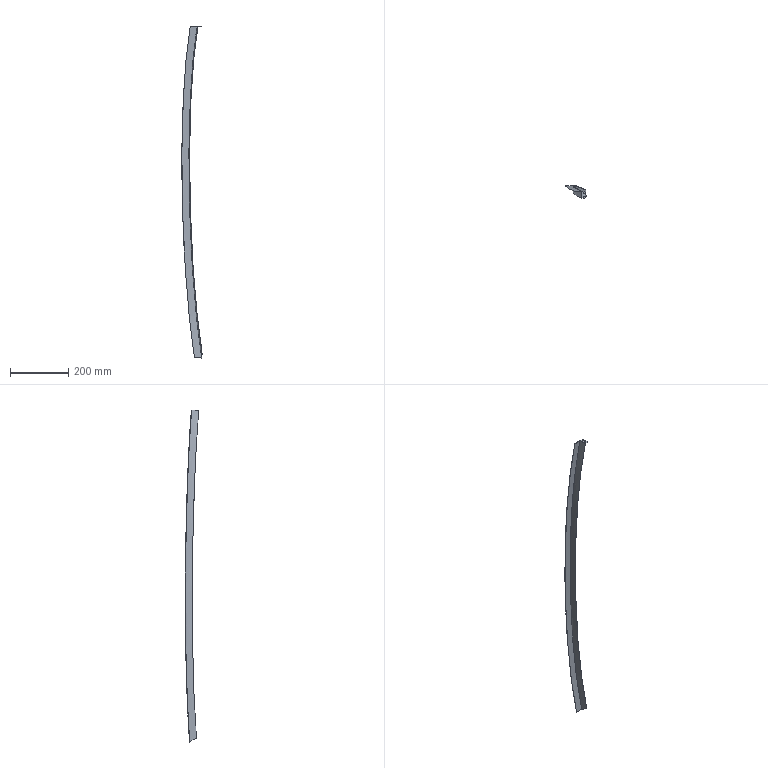Part | SolidWorks | features BaseBody 2 | 2 solids | 19 faces | box 69.762 x 45.708 x 1140 mm | volume 41473 mm3 | plane 10 | spline 5 | cylinder 4 | commonest cylinder face diameters 3.2 x4
STEP:
#1=CARTESIAN_POINT('',(-229.182,136.394,-526.751));
#2=VERTEX_POINT('',#1);
#3=CARTESIAN_POINT('',(-230.802,159.266,-540.095));
#4=VERTEX_POINT('',#3);
#5=CARTESIAN_POINT('',(-229.182,136.394,-526.751));
#6=DIRECTION('',(-0.06105,0.8621,-0.503));
#7=VECTOR('',#6,1000.);
#8=LINE('',#5,#7);
#9=EDGE_CURVE('',#2,#4,#8,.T.);
#10=ORIENTED_EDGE('',*,*,#9,.T.);
#11=CARTESIAN_POINT('',(-255.331,159.266,-540.095));
#12=VERTEX_POINT('',#11);
#13=CARTESIAN_POINT('',(-241.927,159.266,-540.095));
#14=DIRECTION('',(-1.,0.,0.));
#15=VECTOR('',#14,1000.);
#16=LINE('',#13,#15);
#17=EDGE_CURVE('',#4,#12,#16,.T.);
#18=ORIENTED_EDGE('',*,*,#17,.T.);
#19=CARTESIAN_POINT('',(-255.331,159.698,-540.347));
#20=VERTEX_POINT('',#19);
#21=CARTESIAN_POINT('',(-255.331,159.482,-540.221));
#22=DIRECTION('',(0.,-0.8638,0.5039));
#23=VECTOR('',#22,1000.);
#24=LINE('',#21,#23);
#25=EDGE_CURVE('',#20,#12,#24,.T.);
#26=ORIENTED_EDGE('',*,*,#25,.F.);
#27=CARTESIAN_POINT('',(-230.802,159.698,-540.347));
#28=VERTEX_POINT('',#27);
#29=CARTESIAN_POINT('',(-241.927,159.698,-540.347));
#30=DIRECTION('',(1.,0.,0.));
#31=VECTOR('',#30,1000.);
#32=LINE('',#29,#31);
#33=EDGE_CURVE('',#20,#28,#32,.T.);
#34=ORIENTED_EDGE('',*,*,#33,.T.);
#35=CARTESIAN_POINT('',(-230.303,159.292,-540.11));
#36=VERTEX_POINT('',#35);
#37=CARTESIAN_POINT('',(-230.802,159.698,-540.347));
#38=CARTESIAN_POINT('',(-230.739,159.698,-540.347));
#39=CARTESIAN_POINT('',(-230.614,159.677,-540.335));
#40=CARTESIAN_POINT('',(-230.454,159.59,-540.284));
#41=CARTESIAN_POINT('',(-230.34,159.458,-540.207));
#42=CARTESIAN_POINT('',(-230.307,159.349,-540.143));
#43=CARTESIAN_POINT('',(-230.303,159.292,-540.11));
#44=B_SPLINE_CURVE_WITH_KNOTS('',3,(#37,#38,#39,#40,#41,#42,#43),.UNSPECIFIED.,.F.,.F.,(4,1,1,1,4),(0.,0.0001877,0.0003754,0.0005631,0.0007508),.UNSPECIFIED.);
#45=EDGE_CURVE('',#28,#36,#44,.T.);
#46=ORIENTED_EDGE('',*,*,#45,.T.);
#47=CARTESIAN_POINT('',(-228.683,136.42,-526.767));
#48=VERTEX_POINT('',#47);
#49=CARTESIAN_POINT('',(-230.303,159.292,-540.11));
#50=DIRECTION('',(0.06105,-0.8621,0.503));
#51=VECTOR('',#50,1000.);
#52=LINE('',#49,#51);
#53=EDGE_CURVE('',#36,#48,#52,.T.);
#54=ORIENTED_EDGE('',*,*,#53,.T.);
#55=CARTESIAN_POINT('',(-228.933,136.407,-526.759));
#56=DIRECTION('',(0.9981,0.05273,-0.03076));
#57=VECTOR('',#56,1000.);
#58=LINE('',#55,#57);
#59=EDGE_CURVE('',#2,#48,#58,.T.);
#60=ORIENTED_EDGE('',*,*,#59,.F.);
#61=EDGE_LOOP('',(#10,#18,#26,#34,#46,#54,#60));
#62=FACE_OUTER_BOUND('',#61,.T.);
#63=CARTESIAN_POINT('',(-255.331,136.254,-526.67));
#64=DIRECTION('',(0.,-0.5039,-0.8638));
#65=DIRECTION('',(0.,0.8638,-0.5039));
#66=AXIS2_PLACEMENT_3D('',#63,#64,#65);
#67=PLANE('',#66);
#68=ADVANCED_FACE('',(#62),#67,.T.);
#69=ORIENTED_EDGE('',*,*,#17,.F.);
#70=CARTESIAN_POINT('',(-245.765,152.9,599.5));
#71=VERTEX_POINT('',#70);
#72=CARTESIAN_POINT('',(-230.802,159.266,-540.095));
#73=CARTESIAN_POINT('',(-278.517,182.395,-221.327));
#74=CARTESIAN_POINT('',(-291.651,175.741,308.037));
#75=CARTESIAN_POINT('',(-245.765,152.9,599.5));
#76=B_SPLINE_CURVE_WITH_KNOTS('',3,(#72,#73,#74,#75),.UNSPECIFIED.,.F.,.F.,(4,4),(0.,1.),.UNSPECIFIED.);
#77=EDGE_CURVE('',#4,#71,#76,.T.);
#78=ORIENTED_EDGE('',*,*,#77,.T.);
#79=CARTESIAN_POINT('',(-269.86,152.9,599.5));
#80=VERTEX_POINT('',#79);
#81=CARTESIAN_POINT('',(-257.812,152.9,599.5));
#82=DIRECTION('',(-1.,0.,0.));
#83=VECTOR('',#82,1000.);
#84=LINE('',#81,#83);
#85=EDGE_CURVE('',#71,#80,#84,.T.);
#86=ORIENTED_EDGE('',*,*,#85,.T.);
#87=CARTESIAN_POINT('',(-269.86,152.9,599.5));
#88=CARTESIAN_POINT('',(-315.891,175.741,308.037));
#89=CARTESIAN_POINT('',(-302.902,182.395,-221.327));
#90=CARTESIAN_POINT('',(-255.331,159.266,-540.095));
#91=B_SPLINE_CURVE_WITH_KNOTS('',3,(#87,#88,#89,#90),.UNSPECIFIED.,.F.,.F.,(4,4),(0.,1.),.UNSPECIFIED.);
#92=EDGE_CURVE('',#80,#12,#91,.T.);
#93=ORIENTED_EDGE('',*,*,#92,.T.);
#94=EDGE_LOOP('',(#69,#78,#86,#93));
#95=FACE_OUTER_BOUND('',#94,.T.);
#96=CARTESIAN_POINT('',(-245.524,152.9,599.5));
#97=CARTESIAN_POINT('',(-291.408,175.741,308.037));
#98=CARTESIAN_POINT('',(-278.273,182.395,-221.327));
#99=CARTESIAN_POINT('',(-230.556,159.266,-540.095));
#100=CARTESIAN_POINT('',(-245.604,152.9,599.5));
#101=CARTESIAN_POINT('',(-291.489,175.741,308.037));
#102=CARTESIAN_POINT('',(-278.355,182.395,-221.327));
#103=CARTESIAN_POINT('',(-230.638,159.266,-540.095));
#104=CARTESIAN_POINT('',(-245.685,152.9,599.5));
#105=CARTESIAN_POINT('',(-291.57,175.741,308.037));
#106=CARTESIAN_POINT('',(-278.436,182.395,-221.327));
#107=CARTESIAN_POINT('',(-230.72,159.266,-540.095));
#108=CARTESIAN_POINT('',(-245.765,152.9,599.5));
#109=CARTESIAN_POINT('',(-291.651,175.741,308.037));
#110=CARTESIAN_POINT('',(-278.517,182.395,-221.327));
#111=CARTESIAN_POINT('',(-230.802,159.266,-540.095));
#112=CARTESIAN_POINT('',(-247.773,152.9,599.5));
#113=CARTESIAN_POINT('',(-293.671,175.741,308.037));
#114=CARTESIAN_POINT('',(-280.549,182.395,-221.327));
#115=CARTESIAN_POINT('',(-232.846,159.266,-540.095));
#116=CARTESIAN_POINT('',(-251.789,152.9,599.5));
#117=CARTESIAN_POINT('',(-297.711,175.741,308.037));
#118=CARTESIAN_POINT('',(-284.614,182.395,-221.327));
#119=CARTESIAN_POINT('',(-236.934,159.266,-540.095));
#120=CARTESIAN_POINT('',(-257.812,152.9,599.5));
#121=CARTESIAN_POINT('',(-303.771,175.741,308.037));
#122=CARTESIAN_POINT('',(-290.71,182.395,-221.327));
#123=CARTESIAN_POINT('',(-243.067,159.266,-540.095));
#124=CARTESIAN_POINT('',(-263.836,152.9,599.5));
#125=CARTESIAN_POINT('',(-309.831,175.741,308.037));
#126=CARTESIAN_POINT('',(-296.806,182.395,-221.327));
#127=CARTESIAN_POINT('',(-249.199,159.266,-540.095));
#128=CARTESIAN_POINT('',(-267.852,152.9,599.5));
#129=CARTESIAN_POINT('',(-313.871,175.741,308.037));
#130=CARTESIAN_POINT('',(-300.87,182.395,-221.327));
#131=CARTESIAN_POINT('',(-253.287,159.266,-540.095));
#132=CARTESIAN_POINT('',(-269.86,152.9,599.5));
#133=CARTESIAN_POINT('',(-315.891,175.741,308.037));
#134=CARTESIAN_POINT('',(-302.902,182.395,-221.327));
#135=CARTESIAN_POINT('',(-255.331,159.266,-540.095));
#136=CARTESIAN_POINT('',(-269.94,152.9,599.5));
#137=CARTESIAN_POINT('',(-315.971,175.741,308.037));
#138=CARTESIAN_POINT('',(-302.983,182.395,-221.327));
#139=CARTESIAN_POINT('',(-255.413,159.266,-540.095));
#140=CARTESIAN_POINT('',(-270.021,152.9,599.5));
#141=CARTESIAN_POINT('',(-316.052,175.741,308.037));
#142=CARTESIAN_POINT('',(-303.065,182.395,-221.327));
#143=CARTESIAN_POINT('',(-255.495,159.266,-540.095));
#144=CARTESIAN_POINT('',(-270.101,152.9,599.5));
#145=CARTESIAN_POINT('',(-316.133,175.741,308.037));
#146=CARTESIAN_POINT('',(-303.146,182.395,-221.327));
#147=CARTESIAN_POINT('',(-255.577,159.266,-540.095));
#148=B_SPLINE_SURFACE_WITH_KNOTS('',3,3,((#96,#97,#98,#99),(#100,#101,#102,#103),(#104,#105,#106,#107),(#108,#109,#110,#111),(#112,#113,#114,#115),(#116,#117,#118,#119),(#120,#121,#122,#123),(#124,#125,#126,#127),(#128,#129,#130,#131),(#132,#133,#134,#135),(#136,#137,#138,#139),(#140,#141,#142,#143),(#144,#145,#146,#147)),.UNSPECIFIED.,.F.,.F.,.F.,(4,3,1,1,1,3,4),(4,4),(0.7539,0.7562,0.816,0.8757,0.9354,0.9951,0.9975),(0.,1.),.UNSPECIFIED.);
#149=ADVANCED_FACE('',(#95),#148,.T.);
#150=ORIENTED_EDGE('',*,*,#9,.F.);
#151=CARTESIAN_POINT('',(-243.797,128.416,599.5));
#152=VERTEX_POINT('',#151);
#153=CARTESIAN_POINT('',(-229.182,136.394,-526.751));
#154=CARTESIAN_POINT('',(-276.782,158.986,-212.431));
#155=CARTESIAN_POINT('',(-289.799,151.794,312.485));
#156=CARTESIAN_POINT('',(-243.797,128.416,599.5));
#157=B_SPLINE_CURVE_WITH_KNOTS('',3,(#153,#154,#155,#156),.UNSPECIFIED.,.F.,.F.,(4,4),(0.,1.),.UNSPECIFIED.);
#158=EDGE_CURVE('',#2,#152,#157,.T.);
#159=ORIENTED_EDGE('',*,*,#158,.T.);
#160=CARTESIAN_POINT('',(-245.266,152.431,599.5));
#161=VERTEX_POINT('',#160);
#162=CARTESIAN_POINT('',(-245.266,152.431,599.5));
#163=DIRECTION('',(-0.06105,0.9981,0.));
#164=VECTOR('',#163,1000.);
#165=LINE('',#162,#164);
#166=EDGE_CURVE('',#152,#161,#165,.T.);
#167=ORIENTED_EDGE('',*,*,#166,.T.);
#168=CARTESIAN_POINT('',(-245.266,152.431,599.5));
#169=CARTESIAN_POINT('',(-245.27,152.49,599.5));
#170=CARTESIAN_POINT('',(-245.299,152.612,599.5));
#171=CARTESIAN_POINT('',(-245.412,152.771,599.5));
#172=CARTESIAN_POINT('',(-245.577,152.877,599.5));
#173=CARTESIAN_POINT('',(-245.703,152.9,599.5));
#174=CARTESIAN_POINT('',(-245.765,152.9,599.5));
#175=B_SPLINE_CURVE_WITH_KNOTS('',3,(#168,#169,#170,#171,#172,#173,#174),.UNSPECIFIED.,.F.,.F.,(4,1,1,1,4),(0.,0.0001877,0.0003755,0.0005632,0.000751),.UNSPECIFIED.);
#176=EDGE_CURVE('',#161,#71,#175,.T.);
#177=ORIENTED_EDGE('',*,*,#176,.T.);
#178=ORIENTED_EDGE('',*,*,#77,.F.);
#179=EDGE_LOOP('',(#150,#159,#167,#177,#178));
#180=FACE_OUTER_BOUND('',#179,.T.);
#181=CARTESIAN_POINT('',(-243.782,128.169,599.5));
#182=CARTESIAN_POINT('',(-289.783,151.553,312.529));
#183=CARTESIAN_POINT('',(-276.766,158.751,-212.342));
#184=CARTESIAN_POINT('',(-229.166,136.165,-526.618));
#185=CARTESIAN_POINT('',(-243.787,128.251,599.5));
#186=CARTESIAN_POINT('',(-289.789,151.633,312.514));
#187=CARTESIAN_POINT('',(-276.771,158.829,-212.372));
#188=CARTESIAN_POINT('',(-229.171,136.241,-526.662));
#189=CARTESIAN_POINT('',(-243.792,128.334,599.5));
#190=CARTESIAN_POINT('',(-289.794,151.714,312.499));
#191=CARTESIAN_POINT('',(-276.776,158.907,-212.402));
#192=CARTESIAN_POINT('',(-229.177,136.317,-526.707));
#193=CARTESIAN_POINT('',(-243.797,128.416,599.5));
#194=CARTESIAN_POINT('',(-289.799,151.794,312.485));
#195=CARTESIAN_POINT('',(-276.782,158.986,-212.431));
#196=CARTESIAN_POINT('',(-229.182,136.394,-526.751));
#197=CARTESIAN_POINT('',(-243.92,130.419,599.5));
#198=CARTESIAN_POINT('',(-289.924,153.747,312.125));
#199=CARTESIAN_POINT('',(-276.91,160.888,-213.152));
#200=CARTESIAN_POINT('',(-229.313,138.246,-527.832));
#201=CARTESIAN_POINT('',(-244.164,134.421,599.5));
#202=CARTESIAN_POINT('',(-290.175,157.65,311.404));
#203=CARTESIAN_POINT('',(-277.166,164.693,-214.593));
#204=CARTESIAN_POINT('',(-229.576,141.952,-529.994));
#205=CARTESIAN_POINT('',(-244.531,140.421,599.5));
#206=CARTESIAN_POINT('',(-290.551,163.505,310.322));
#207=CARTESIAN_POINT('',(-277.551,170.402,-216.757));
#208=CARTESIAN_POINT('',(-229.97,147.515,-533.24));
#209=CARTESIAN_POINT('',(-244.898,146.422,599.5));
#210=CARTESIAN_POINT('',(-290.927,169.359,309.24));
#211=CARTESIAN_POINT('',(-277.936,176.11,-218.92));
#212=CARTESIAN_POINT('',(-230.364,153.077,-536.485));
#213=CARTESIAN_POINT('',(-245.143,150.426,599.5));
#214=CARTESIAN_POINT('',(-291.178,173.264,308.52));
#215=CARTESIAN_POINT('',(-278.193,179.915,-220.361));
#216=CARTESIAN_POINT('',(-230.626,156.782,-538.646));
#217=CARTESIAN_POINT('',(-245.27,152.49,599.5));
#218=CARTESIAN_POINT('',(-291.307,175.275,308.149));
#219=CARTESIAN_POINT('',(-278.325,181.873,-221.103));
#220=CARTESIAN_POINT('',(-230.761,158.688,-539.758));
#221=CARTESIAN_POINT('',(-245.299,152.612,599.5));
#222=CARTESIAN_POINT('',(-291.329,175.392,308.128));
#223=CARTESIAN_POINT('',(-278.34,181.986,-221.144));
#224=CARTESIAN_POINT('',(-230.768,158.795,-539.82));
#225=CARTESIAN_POINT('',(-245.412,152.771,599.5));
#226=CARTESIAN_POINT('',(-291.408,175.55,308.098));
#227=CARTESIAN_POINT('',(-278.385,182.143,-221.205));
#228=CARTESIAN_POINT('',(-230.779,158.951,-539.911));
#229=CARTESIAN_POINT('',(-245.577,152.877,599.5));
#230=CARTESIAN_POINT('',(-291.522,175.672,308.068));
#231=CARTESIAN_POINT('',(-278.447,182.281,-221.265));
#232=CARTESIAN_POINT('',(-230.79,159.106,-540.002));
#233=CARTESIAN_POINT('',(-245.703,152.9,599.5));
#234=CARTESIAN_POINT('',(-291.608,175.723,308.047));
#235=CARTESIAN_POINT('',(-278.494,182.359,-221.306));
#236=CARTESIAN_POINT('',(-230.798,159.212,-540.063));
#237=CARTESIAN_POINT('',(-245.765,152.9,599.5));
#238=CARTESIAN_POINT('',(-291.651,175.741,308.037));
#239=CARTESIAN_POINT('',(-278.517,182.395,-221.327));
#240=CARTESIAN_POINT('',(-230.802,159.266,-540.095));
#241=B_SPLINE_SURFACE_WITH_KNOTS('',3,3,((#181,#182,#183,#184),(#185,#186,#187,#188),(#189,#190,#191,#192),(#193,#194,#195,#196),(#197,#198,#199,#200),(#201,#202,#203,#204),(#205,#206,#207,#208),(#209,#210,#211,#212),(#213,#214,#215,#216),(#217,#218,#219,#220),(#221,#222,#223,#224),(#225,#226,#227,#228),(#229,#230,#231,#232),(#233,#234,#235,#236),(#237,#238,#239,#240)),.UNSPECIFIED.,.F.,.F.,.F.,(4,3,1,1,1,2,1,1,1,4),(4,4),(0.5017,0.5042,0.5654,0.6266,0.6877,0.7489,0.7508,0.7526,0.7544,0.7562),(0.,1.),.UNSPECIFIED.);
#242=ADVANCED_FACE('',(#180),#241,.T.);
#243=ORIENTED_EDGE('',*,*,#33,.F.);
#244=CARTESIAN_POINT('',(-269.86,153.4,599.5));
#245=VERTEX_POINT('',#244);
#246=CARTESIAN_POINT('',(-255.331,159.698,-540.347));
#247=CARTESIAN_POINT('',(-302.902,182.85,-221.495));
#248=CARTESIAN_POINT('',(-315.891,176.218,307.953));
#249=CARTESIAN_POINT('',(-269.86,153.4,599.5));
#250=B_SPLINE_CURVE_WITH_KNOTS('',3,(#246,#247,#248,#249),.UNSPECIFIED.,.F.,.F.,(4,4),(0.,1.),.UNSPECIFIED.);
#251=EDGE_CURVE('',#20,#245,#250,.T.);
#252=ORIENTED_EDGE('',*,*,#251,.T.);
#253=CARTESIAN_POINT('',(-245.295,153.4,599.5));
#254=VERTEX_POINT('',#253);
#255=CARTESIAN_POINT('',(-243.139,153.4,599.5));
#256=DIRECTION('',(1.,0.,0.));
#257=VECTOR('',#256,1000.);
#258=LINE('',#255,#257);
#259=EDGE_CURVE('',#245,#254,#258,.T.);
#260=ORIENTED_EDGE('',*,*,#259,.T.);
#261=CARTESIAN_POINT('',(-244.796,152.931,599.5));
#262=VERTEX_POINT('',#261);
#263=CARTESIAN_POINT('',(-245.295,153.4,599.5));
#264=CARTESIAN_POINT('',(-245.232,153.4,599.5));
#265=CARTESIAN_POINT('',(-245.105,153.376,599.5));
#266=CARTESIAN_POINT('',(-244.941,153.27,599.5));
#267=CARTESIAN_POINT('',(-244.829,153.113,599.5));
#268=CARTESIAN_POINT('',(-244.799,152.991,599.5));
#269=CARTESIAN_POINT('',(-244.796,152.931,599.5));
#270=B_SPLINE_CURVE_WITH_KNOTS('',3,(#263,#264,#265,#266,#267,#268,#269),.UNSPECIFIED.,.F.,.F.,(4,1,1,1,4),(0.,0.0001877,0.0003755,0.0005632,0.000751),.UNSPECIFIED.);
#271=EDGE_CURVE('',#254,#262,#270,.T.);
#272=ORIENTED_EDGE('',*,*,#271,.T.);
#273=CARTESIAN_POINT('',(-243.298,128.447,599.5));
#274=VERTEX_POINT('',#273);
#275=CARTESIAN_POINT('',(-243.298,128.447,599.5));
#276=DIRECTION('',(0.06105,-0.9981,0.));
#277=VECTOR('',#276,1000.);
#278=LINE('',#275,#277);
#279=EDGE_CURVE('',#262,#274,#278,.T.);
#280=ORIENTED_EDGE('',*,*,#279,.T.);
#281=CARTESIAN_POINT('',(-243.298,128.447,599.5));
#282=CARTESIAN_POINT('',(-289.3,151.823,312.48));
#283=CARTESIAN_POINT('',(-276.283,159.013,-212.442));
#284=CARTESIAN_POINT('',(-228.683,136.42,-526.767));
#285=B_SPLINE_CURVE_WITH_KNOTS('',3,(#281,#282,#283,#284),.UNSPECIFIED.,.F.,.F.,(4,4),(0.,1.),.UNSPECIFIED.);
#286=EDGE_CURVE('',#274,#48,#285,.T.);
#287=ORIENTED_EDGE('',*,*,#286,.T.);
#288=ORIENTED_EDGE('',*,*,#53,.F.);
#289=ORIENTED_EDGE('',*,*,#45,.F.);
#290=EDGE_LOOP('',(#243,#252,#260,#272,#280,#287,#288,#289));
#291=FACE_OUTER_BOUND('',#290,.T.);
#292=CARTESIAN_POINT('',(-269.86,153.4,599.5));
#293=CARTESIAN_POINT('',(-315.891,176.218,307.953));
#294=CARTESIAN_POINT('',(-302.902,182.85,-221.495));
#295=CARTESIAN_POINT('',(-255.331,159.698,-540.347));
#296=CARTESIAN_POINT('',(-267.813,153.4,599.5));
#297=CARTESIAN_POINT('',(-313.844,176.218,307.953));
#298=CARTESIAN_POINT('',(-300.857,182.85,-221.495));
#299=CARTESIAN_POINT('',(-253.287,159.698,-540.347));
#300=CARTESIAN_POINT('',(-263.719,153.4,599.5));
#301=CARTESIAN_POINT('',(-309.752,176.218,307.953));
#302=CARTESIAN_POINT('',(-296.767,182.85,-221.495));
#303=CARTESIAN_POINT('',(-249.199,159.698,-540.347));
#304=CARTESIAN_POINT('',(-257.577,153.4,599.5));
#305=CARTESIAN_POINT('',(-303.614,176.218,307.953));
#306=CARTESIAN_POINT('',(-290.631,182.85,-221.495));
#307=CARTESIAN_POINT('',(-243.067,159.698,-540.347));
#308=CARTESIAN_POINT('',(-251.436,153.4,599.5));
#309=CARTESIAN_POINT('',(-297.475,176.218,307.953));
#310=CARTESIAN_POINT('',(-284.496,182.85,-221.495));
#311=CARTESIAN_POINT('',(-236.934,159.698,-540.347));
#312=CARTESIAN_POINT('',(-247.342,153.4,599.5));
#313=CARTESIAN_POINT('',(-293.383,176.218,307.953));
#314=CARTESIAN_POINT('',(-280.406,182.85,-221.495));
#315=CARTESIAN_POINT('',(-232.846,159.698,-540.347));
#316=CARTESIAN_POINT('',(-245.232,153.4,599.5));
#317=CARTESIAN_POINT('',(-291.274,176.218,307.953));
#318=CARTESIAN_POINT('',(-278.298,182.85,-221.495));
#319=CARTESIAN_POINT('',(-230.739,159.698,-540.347));
#320=CARTESIAN_POINT('',(-245.105,153.376,599.5));
#321=CARTESIAN_POINT('',(-291.148,176.195,307.957));
#322=CARTESIAN_POINT('',(-278.172,182.828,-221.487));
#323=CARTESIAN_POINT('',(-230.614,159.677,-540.335));
#324=CARTESIAN_POINT('',(-244.941,153.27,599.5));
#325=CARTESIAN_POINT('',(-290.985,176.096,307.974));
#326=CARTESIAN_POINT('',(-278.011,182.735,-221.453));
#327=CARTESIAN_POINT('',(-230.454,159.59,-540.284));
#328=CARTESIAN_POINT('',(-244.829,153.113,599.5));
#329=CARTESIAN_POINT('',(-290.873,175.947,307.999));
#330=CARTESIAN_POINT('',(-277.898,182.594,-221.402));
#331=CARTESIAN_POINT('',(-230.34,159.458,-540.207));
#332=CARTESIAN_POINT('',(-244.799,152.991,599.5));
#333=CARTESIAN_POINT('',(-290.842,175.829,308.021));
#334=CARTESIAN_POINT('',(-277.865,182.481,-221.359));
#335=CARTESIAN_POINT('',(-230.307,159.349,-540.143));
#336=CARTESIAN_POINT('',(-244.671,150.888,599.5));
#337=CARTESIAN_POINT('',(-290.71,173.774,308.402));
#338=CARTESIAN_POINT('',(-277.73,180.473,-220.597));
#339=CARTESIAN_POINT('',(-230.168,157.388,-539.));
#340=CARTESIAN_POINT('',(-244.421,146.806,599.5));
#341=CARTESIAN_POINT('',(-290.453,169.782,309.143));
#342=CARTESIAN_POINT('',(-277.467,176.572,-219.115));
#343=CARTESIAN_POINT('',(-229.898,153.578,-536.776));
#344=CARTESIAN_POINT('',(-244.047,140.687,599.5));
#345=CARTESIAN_POINT('',(-290.069,163.796,310.255));
#346=CARTESIAN_POINT('',(-277.072,170.719,-216.89));
#347=CARTESIAN_POINT('',(-229.493,147.857,-533.439));
#348=CARTESIAN_POINT('',(-243.673,134.57,599.5));
#349=CARTESIAN_POINT('',(-289.684,157.811,311.368));
#350=CARTESIAN_POINT('',(-276.677,164.865,-214.665));
#351=CARTESIAN_POINT('',(-229.088,142.136,-530.101));
#352=CARTESIAN_POINT('',(-243.423,130.489,599.5));
#353=CARTESIAN_POINT('',(-289.428,153.82,312.109));
#354=CARTESIAN_POINT('',(-276.414,160.964,-213.183));
#355=CARTESIAN_POINT('',(-228.818,138.325,-527.878));
#356=CARTESIAN_POINT('',(-243.298,128.447,599.5));
#357=CARTESIAN_POINT('',(-289.3,151.823,312.48));
#358=CARTESIAN_POINT('',(-276.283,159.013,-212.442));
#359=CARTESIAN_POINT('',(-228.683,136.42,-526.767));
#360=B_SPLINE_SURFACE_WITH_KNOTS('',3,3,((#292,#293,#294,#295),(#296,#297,#298,#299),(#300,#301,#302,#303),(#304,#305,#306,#307),(#308,#309,#310,#311),(#312,#313,#314,#315),(#316,#317,#318,#319),(#320,#321,#322,#323),(#324,#325,#326,#327),(#328,#329,#330,#331),(#332,#333,#334,#335),(#336,#337,#338,#339),(#340,#341,#342,#343),(#344,#345,#346,#347),(#348,#349,#350,#351),(#352,#353,#354,#355),(#356,#357,#358,#359)),.UNSPECIFIED.,.F.,.F.,.F.,(4,1,1,1,2,1,1,1,2,1,1,1,4),(4,4),(0.,0.0603,0.1206,0.1809,0.2412,0.2431,0.2449,0.2468,0.2486,0.3113,0.3739,0.4366,0.4993),(0.,1.),.UNSPECIFIED.);
#361=ADVANCED_FACE('',(#291),#360,.T.);
#362=ORIENTED_EDGE('',*,*,#25,.T.);
#363=ORIENTED_EDGE('',*,*,#92,.F.);
#364=CARTESIAN_POINT('',(-269.86,153.15,599.5));
#365=DIRECTION('',(0.,1.,0.));
#366=VECTOR('',#365,1000.);
#367=LINE('',#364,#366);
#368=EDGE_CURVE('',#80,#245,#367,.T.);
#369=ORIENTED_EDGE('',*,*,#368,.T.);
#370=ORIENTED_EDGE('',*,*,#251,.F.);
#371=EDGE_LOOP('',(#362,#363,#369,#370));
#372=FACE_OUTER_BOUND('',#371,.T.);
#373=CARTESIAN_POINT('',(-269.86,152.9,599.5));
#374=CARTESIAN_POINT('',(-315.891,175.741,308.037));
#375=CARTESIAN_POINT('',(-302.902,182.395,-221.327));
#376=CARTESIAN_POINT('',(-255.331,159.266,-540.095));
#377=CARTESIAN_POINT('',(-269.86,152.942,599.5));
#378=CARTESIAN_POINT('',(-315.891,175.781,308.03));
#379=CARTESIAN_POINT('',(-302.902,182.433,-221.341));
#380=CARTESIAN_POINT('',(-255.331,159.302,-540.116));
#381=CARTESIAN_POINT('',(-269.86,153.025,599.5));
#382=CARTESIAN_POINT('',(-315.891,175.86,308.016));
#383=CARTESIAN_POINT('',(-302.902,182.509,-221.369));
#384=CARTESIAN_POINT('',(-255.331,159.374,-540.158));
#385=CARTESIAN_POINT('',(-269.86,153.15,599.5));
#386=CARTESIAN_POINT('',(-315.891,175.98,307.995));
#387=CARTESIAN_POINT('',(-302.902,182.623,-221.411));
#388=CARTESIAN_POINT('',(-255.331,159.482,-540.221));
#389=CARTESIAN_POINT('',(-269.86,153.275,599.5));
#390=CARTESIAN_POINT('',(-315.891,176.099,307.974));
#391=CARTESIAN_POINT('',(-302.902,182.736,-221.453));
#392=CARTESIAN_POINT('',(-255.331,159.59,-540.284));
#393=CARTESIAN_POINT('',(-269.86,153.358,599.5));
#394=CARTESIAN_POINT('',(-315.891,176.179,307.96));
#395=CARTESIAN_POINT('',(-302.902,182.812,-221.481));
#396=CARTESIAN_POINT('',(-255.331,159.662,-540.326));
#397=CARTESIAN_POINT('',(-269.86,153.4,599.5));
#398=CARTESIAN_POINT('',(-315.891,176.218,307.953));
#399=CARTESIAN_POINT('',(-302.902,182.85,-221.495));
#400=CARTESIAN_POINT('',(-255.331,159.698,-540.347));
#401=B_SPLINE_SURFACE_WITH_KNOTS('',3,3,((#373,#374,#375,#376),(#377,#378,#379,#380),(#381,#382,#383,#384),(#385,#386,#387,#388),(#389,#390,#391,#392),(#393,#394,#395,#396),(#397,#398,#399,#400)),.UNSPECIFIED.,.F.,.F.,.F.,(4,1,1,1,4),(4,4),(0.9951,0.9963,0.9975,0.9988,1.),(0.,1.),.UNSPECIFIED.);
#402=ADVANCED_FACE('',(#372),#401,.T.);
#403=ORIENTED_EDGE('',*,*,#85,.F.);
#404=ORIENTED_EDGE('',*,*,#176,.F.);
#405=ORIENTED_EDGE('',*,*,#166,.F.);
#406=CARTESIAN_POINT('',(-243.797,128.416,599.5));
#407=DIRECTION('',(-0.9981,-0.06105,0.));
#408=VECTOR('',#407,1000.);
#409=LINE('',#406,#408);
#410=EDGE_CURVE('',#274,#152,#409,.T.);
#411=ORIENTED_EDGE('',*,*,#410,.F.);
#412=ORIENTED_EDGE('',*,*,#279,.F.);
#413=ORIENTED_EDGE('',*,*,#271,.F.);
#414=ORIENTED_EDGE('',*,*,#259,.F.);
#415=ORIENTED_EDGE('',*,*,#368,.F.);
#416=EDGE_LOOP('',(#403,#404,#405,#411,#412,#413,#414,#415));
#417=FACE_OUTER_BOUND('',#416,.T.);
#418=CARTESIAN_POINT('',(-243.139,128.266,599.5));
#419=DIRECTION('',(0.,0.,-1.));
#420=DIRECTION('',(-1.,0.,0.));
#421=AXIS2_PLACEMENT_3D('',#418,#419,#420);
#422=PLANE('',#421);
#423=ADVANCED_FACE('',(#417),#422,.F.);
#424=ORIENTED_EDGE('',*,*,#59,.T.);
#425=ORIENTED_EDGE('',*,*,#286,.F.);
#426=ORIENTED_EDGE('',*,*,#410,.T.);
#427=ORIENTED_EDGE('',*,*,#158,.F.);
#428=EDGE_LOOP('',(#424,#425,#426,#427));
#429=FACE_OUTER_BOUND('',#428,.T.);
#430=CARTESIAN_POINT('',(-243.298,128.447,599.5));
#431=CARTESIAN_POINT('',(-289.3,151.823,312.48));
#432=CARTESIAN_POINT('',(-276.283,159.013,-212.442));
#433=CARTESIAN_POINT('',(-228.683,136.42,-526.767));
#434=CARTESIAN_POINT('',(-243.34,128.444,599.5));
#435=CARTESIAN_POINT('',(-289.341,151.821,312.48));
#436=CARTESIAN_POINT('',(-276.324,159.011,-212.441));
#437=CARTESIAN_POINT('',(-228.725,136.418,-526.765));
#438=CARTESIAN_POINT('',(-243.423,128.439,599.5));
#439=CARTESIAN_POINT('',(-289.425,151.816,312.481));
#440=CARTESIAN_POINT('',(-276.407,159.007,-212.439));
#441=CARTESIAN_POINT('',(-228.808,136.413,-526.763));
#442=CARTESIAN_POINT('',(-243.548,128.431,599.5));
#443=CARTESIAN_POINT('',(-289.549,151.809,312.482));
#444=CARTESIAN_POINT('',(-276.532,159.,-212.437));
#445=CARTESIAN_POINT('',(-228.933,136.407,-526.759));
#446=CARTESIAN_POINT('',(-243.672,128.424,599.5));
#447=CARTESIAN_POINT('',(-289.674,151.802,312.483));
#448=CARTESIAN_POINT('',(-276.657,158.993,-212.434));
#449=CARTESIAN_POINT('',(-229.057,136.4,-526.755));
#450=CARTESIAN_POINT('',(-243.756,128.419,599.5));
#451=CARTESIAN_POINT('',(-289.757,151.797,312.484));
#452=CARTESIAN_POINT('',(-276.74,158.988,-212.432));
#453=CARTESIAN_POINT('',(-229.141,136.396,-526.752));
#454=CARTESIAN_POINT('',(-243.797,128.416,599.5));
#455=CARTESIAN_POINT('',(-289.799,151.794,312.485));
#456=CARTESIAN_POINT('',(-276.782,158.986,-212.431));
#457=CARTESIAN_POINT('',(-229.182,136.394,-526.751));
#458=B_SPLINE_SURFACE_WITH_KNOTS('',3,3,((#430,#431,#432,#433),(#434,#435,#436,#437),(#438,#439,#440,#441),(#442,#443,#444,#445),(#446,#447,#448,#449),(#450,#451,#452,#453),(#454,#455,#456,#457)),.UNSPECIFIED.,.F.,.F.,.F.,(4,1,1,1,4),(4,4),(0.4993,0.5005,0.5017,0.5029,0.5042),(0.,1.),.UNSPECIFIED.);
#459=ADVANCED_FACE('',(#429),#458,.T.);
#460=CLOSED_SHELL('',(#68,#149,#242,#361,#402,#423,#459));
#461=MANIFOLD_SOLID_BREP('',#460);
#462=CARTESIAN_POINT('',(-235.817,134.447,599.));
#463=VERTEX_POINT('',#462);
#464=CARTESIAN_POINT('',(-239.017,134.447,599.));
#465=VERTEX_POINT('',#464);
#466=CARTESIAN_POINT('',(-237.417,134.447,599.));
#467=DIRECTION('',(0.,0.,-1.));
#468=DIRECTION('',(1.,0.,0.));
#469=AXIS2_PLACEMENT_3D('',#466,#467,#468);
#470=CIRCLE('',#469,1.6);
#471=EDGE_CURVE('',#463,#465,#470,.T.);
#472=ORIENTED_EDGE('',*,*,#471,.T.);
#473=CARTESIAN_POINT('',(-239.017,134.447,599.5));
#474=VERTEX_POINT('',#473);
#475=CARTESIAN_POINT('',(-239.017,134.447,599.));
#476=DIRECTION('',(0.,0.,1.));
#477=VECTOR('',#476,1000.);
#478=LINE('',#475,#477);
#479=EDGE_CURVE('',#465,#474,#478,.T.);
#480=ORIENTED_EDGE('',*,*,#479,.T.);
#481=CARTESIAN_POINT('',(-235.817,134.447,599.5));
#482=VERTEX_POINT('',#481);
#483=CARTESIAN_POINT('',(-237.417,134.447,599.5));
#484=DIRECTION('',(0.,0.,1.));
#485=DIRECTION('',(1.,0.,0.));
#486=AXIS2_PLACEMENT_3D('',#483,#484,#485);
#487=CIRCLE('',#486,1.6);
#488=EDGE_CURVE('',#474,#482,#487,.T.);
#489=ORIENTED_EDGE('',*,*,#488,.T.);
#490=CARTESIAN_POINT('',(-235.817,134.447,599.));
#491=DIRECTION('',(0.,0.,1.));
#492=VECTOR('',#491,1000.);
#493=LINE('',#490,#492);
#494=EDGE_CURVE('',#463,#482,#493,.T.);
#495=ORIENTED_EDGE('',*,*,#494,.F.);
#496=EDGE_LOOP('',(#472,#480,#489,#495));
#497=FACE_OUTER_BOUND('',#496,.T.);
#498=CARTESIAN_POINT('',(-237.417,134.447,599.));
#499=DIRECTION('',(0.,0.,1.));
#500=DIRECTION('',(1.,0.,0.));
#501=AXIS2_PLACEMENT_3D('',#498,#499,#500);
#502=CYLINDRICAL_SURFACE('',#501,1.6);
#503=ADVANCED_FACE('',(#497),#502,.F.);
#504=CARTESIAN_POINT('',(-235.817,146.394,599.));
#505=VERTEX_POINT('',#504);
#506=CARTESIAN_POINT('',(-239.017,146.394,599.));
#507=VERTEX_POINT('',#506);
#508=CARTESIAN_POINT('',(-237.417,146.394,599.));
#509=DIRECTION('',(0.,0.,-1.));
#510=DIRECTION('',(1.,0.,0.));
#511=AXIS2_PLACEMENT_3D('',#508,#509,#510);
#512=CIRCLE('',#511,1.6);
#513=EDGE_CURVE('',#505,#507,#512,.T.);
#514=ORIENTED_EDGE('',*,*,#513,.T.);
#515=CARTESIAN_POINT('',(-239.017,146.394,599.5));
#516=VERTEX_POINT('',#515);
#517=CARTESIAN_POINT('',(-239.017,146.394,599.));
#518=DIRECTION('',(0.,0.,1.));
#519=VECTOR('',#518,1000.);
#520=LINE('',#517,#519);
#521=EDGE_CURVE('',#507,#516,#520,.T.);
#522=ORIENTED_EDGE('',*,*,#521,.T.);
#523=CARTESIAN_POINT('',(-235.817,146.394,599.5));
#524=VERTEX_POINT('',#523);
#525=CARTESIAN_POINT('',(-237.417,146.394,599.5));
#526=DIRECTION('',(0.,0.,-1.));
#527=DIRECTION('',(1.,0.,0.));
#528=AXIS2_PLACEMENT_3D('',#525,#526,#527);
#529=CIRCLE('',#528,1.6);
#530=EDGE_CURVE('',#524,#516,#529,.T.);
#531=ORIENTED_EDGE('',*,*,#530,.F.);
#532=CARTESIAN_POINT('',(-235.817,146.394,599.));
#533=DIRECTION('',(0.,0.,1.));
#534=VECTOR('',#533,1000.);
#535=LINE('',#532,#534);
#536=EDGE_CURVE('',#505,#524,#535,.T.);
#537=ORIENTED_EDGE('',*,*,#536,.F.);
#538=EDGE_LOOP('',(#514,#522,#531,#537));
#539=FACE_OUTER_BOUND('',#538,.T.);
#540=CARTESIAN_POINT('',(-237.417,146.394,599.));
#541=DIRECTION('',(0.,0.,1.));
#542=DIRECTION('',(1.,0.,0.));
#543=AXIS2_PLACEMENT_3D('',#540,#541,#542);
#544=CYLINDRICAL_SURFACE('',#543,1.6);
#545=ADVANCED_FACE('',(#539),#544,.F.);
#546=ORIENTED_EDGE('',*,*,#479,.F.);
#547=CARTESIAN_POINT('',(-237.417,134.447,599.));
#548=DIRECTION('',(0.,0.,-1.));
#549=DIRECTION('',(1.,0.,0.));
#550=AXIS2_PLACEMENT_3D('',#547,#548,#549);
#551=CIRCLE('',#550,1.6);
#552=EDGE_CURVE('',#465,#463,#551,.T.);
#553=ORIENTED_EDGE('',*,*,#552,.T.);
#554=ORIENTED_EDGE('',*,*,#494,.T.);
#555=CARTESIAN_POINT('',(-237.417,134.447,599.5));
#556=DIRECTION('',(0.,0.,1.));
#557=DIRECTION('',(1.,0.,0.));
#558=AXIS2_PLACEMENT_3D('',#555,#556,#557);
#559=CIRCLE('',#558,1.6);
#560=EDGE_CURVE('',#482,#474,#559,.T.);
#561=ORIENTED_EDGE('',*,*,#560,.T.);
#562=EDGE_LOOP('',(#546,#553,#554,#561));
#563=FACE_OUTER_BOUND('',#562,.T.);
#564=CARTESIAN_POINT('',(-237.417,134.447,599.));
#565=DIRECTION('',(0.,0.,1.));
#566=DIRECTION('',(1.,0.,0.));
#567=AXIS2_PLACEMENT_3D('',#564,#565,#566);
#568=CYLINDRICAL_SURFACE('',#567,1.6);
#569=ADVANCED_FACE('',(#563),#568,.F.);
#570=ORIENTED_EDGE('',*,*,#560,.F.);
#571=ORIENTED_EDGE('',*,*,#488,.F.);
#572=EDGE_LOOP('',(#570,#571));
#573=FACE_BOUND('',#572,.T.);
#574=ORIENTED_EDGE('',*,*,#530,.T.);
#575=CARTESIAN_POINT('',(-237.417,146.394,599.5));
#576=DIRECTION('',(0.,0.,-1.));
#577=DIRECTION('',(1.,0.,0.));
#578=AXIS2_PLACEMENT_3D('',#575,#576,#577);
#579=CIRCLE('',#578,1.6);
#580=EDGE_CURVE('',#516,#524,#579,.T.);
#581=ORIENTED_EDGE('',*,*,#580,.T.);
#582=EDGE_LOOP('',(#574,#581));
#583=FACE_BOUND('',#582,.T.);
#584=CARTESIAN_POINT('',(-235.417,152.394,599.5));
#585=VERTEX_POINT('',#584);
#586=CARTESIAN_POINT('',(-244.763,152.394,599.5));
#587=VERTEX_POINT('',#586);
#588=CARTESIAN_POINT('',(-238.13,152.394,599.5));
#589=DIRECTION('',(-1.,0.,0.));
#590=VECTOR('',#589,1000.);
#591=LINE('',#588,#590);
#592=EDGE_CURVE('',#585,#587,#591,.T.);
#593=ORIENTED_EDGE('',*,*,#592,.T.);
#594=CARTESIAN_POINT('',(-243.298,128.447,599.5));
#595=VERTEX_POINT('',#594);
#596=CARTESIAN_POINT('',(-244.763,152.394,599.5));
#597=DIRECTION('',(0.06105,-0.9981,0.));
#598=VECTOR('',#597,1000.);
#599=LINE('',#596,#598);
#600=EDGE_CURVE('',#587,#595,#599,.T.);
#601=ORIENTED_EDGE('',*,*,#600,.T.);
#602=CARTESIAN_POINT('',(-235.417,128.447,599.5));
#603=VERTEX_POINT('',#602);
#604=CARTESIAN_POINT('',(-238.13,128.447,599.5));
#605=DIRECTION('',(1.,0.,0.));
#606=VECTOR('',#605,1000.);
#607=LINE('',#604,#606);
#608=EDGE_CURVE('',#595,#603,#607,.T.);
#609=ORIENTED_EDGE('',*,*,#608,.T.);
#610=CARTESIAN_POINT('',(-231.417,132.447,599.5));
#611=VERTEX_POINT('',#610);
#612=CARTESIAN_POINT('',(-235.417,128.447,599.5));
#613=DIRECTION('',(0.7071,0.7071,0.));
#614=VECTOR('',#613,1000.);
#615=LINE('',#612,#614);
#616=EDGE_CURVE('',#603,#611,#615,.T.);
#617=ORIENTED_EDGE('',*,*,#616,.T.);
#618=CARTESIAN_POINT('',(-231.417,148.394,599.5));
#619=VERTEX_POINT('',#618);
#620=CARTESIAN_POINT('',(-231.417,140.42,599.5));
#621=DIRECTION('',(0.,1.,0.));
#622=VECTOR('',#621,1000.);
#623=LINE('',#620,#622);
#624=EDGE_CURVE('',#611,#619,#623,.T.);
#625=ORIENTED_EDGE('',*,*,#624,.T.);
#626=CARTESIAN_POINT('',(-231.417,148.394,599.5));
#627=DIRECTION('',(-0.7071,0.7071,0.));
#628=VECTOR('',#627,1000.);
#629=LINE('',#626,#628);
#630=EDGE_CURVE('',#619,#585,#629,.T.);
#631=ORIENTED_EDGE('',*,*,#630,.T.);
#632=EDGE_LOOP('',(#593,#601,#609,#617,#625,#631));
#633=FACE_OUTER_BOUND('',#632,.T.);
#634=CARTESIAN_POINT('',(-244.843,128.447,599.5));
#635=DIRECTION('',(0.,0.,1.));
#636=DIRECTION('',(1.,0.,0.));
#637=AXIS2_PLACEMENT_3D('',#634,#635,#636);
#638=PLANE('',#637);
#639=ADVANCED_FACE('',(#573,#583,#633),#638,.T.);
#640=ORIENTED_EDGE('',*,*,#471,.F.);
#641=ORIENTED_EDGE('',*,*,#552,.F.);
#642=EDGE_LOOP('',(#640,#641));
#643=FACE_BOUND('',#642,.T.);
#644=ORIENTED_EDGE('',*,*,#513,.F.);
#645=CARTESIAN_POINT('',(-237.417,146.394,599.));
#646=DIRECTION('',(0.,0.,-1.));
#647=DIRECTION('',(1.,0.,0.));
#648=AXIS2_PLACEMENT_3D('',#645,#646,#647);
#649=CIRCLE('',#648,1.6);
#650=EDGE_CURVE('',#507,#505,#649,.T.);
#651=ORIENTED_EDGE('',*,*,#650,.F.);
#652=EDGE_LOOP('',(#644,#651));
#653=FACE_BOUND('',#652,.T.);
#654=CARTESIAN_POINT('',(-235.417,128.447,599.));
#655=VERTEX_POINT('',#654);
#656=CARTESIAN_POINT('',(-231.417,132.447,599.));
#657=VERTEX_POINT('',#656);
#658=CARTESIAN_POINT('',(-231.417,132.447,599.));
#659=DIRECTION('',(0.7071,0.7071,0.));
#660=VECTOR('',#659,1000.);
#661=LINE('',#658,#660);
#662=EDGE_CURVE('',#655,#657,#661,.T.);
#663=ORIENTED_EDGE('',*,*,#662,.F.);
#664=CARTESIAN_POINT('',(-243.298,128.447,599.));
#665=VERTEX_POINT('',#664);
#666=CARTESIAN_POINT('',(-238.13,128.447,599.));
#667=DIRECTION('',(1.,0.,0.));
#668=VECTOR('',#667,1000.);
#669=LINE('',#666,#668);
#670=EDGE_CURVE('',#665,#655,#669,.T.);
#671=ORIENTED_EDGE('',*,*,#670,.F.);
#672=CARTESIAN_POINT('',(-244.763,152.394,599.));
#673=VERTEX_POINT('',#672);
#674=CARTESIAN_POINT('',(-243.298,128.447,599.));
#675=DIRECTION('',(0.06105,-0.9981,0.));
#676=VECTOR('',#675,1000.);
#677=LINE('',#674,#676);
#678=EDGE_CURVE('',#673,#665,#677,.T.);
#679=ORIENTED_EDGE('',*,*,#678,.F.);
#680=CARTESIAN_POINT('',(-235.417,152.394,599.));
#681=VERTEX_POINT('',#680);
#682=CARTESIAN_POINT('',(-238.13,152.394,599.));
#683=DIRECTION('',(-1.,0.,0.));
#684=VECTOR('',#683,1000.);
#685=LINE('',#682,#684);
#686=EDGE_CURVE('',#681,#673,#685,.T.);
#687=ORIENTED_EDGE('',*,*,#686,.F.);
#688=CARTESIAN_POINT('',(-231.417,148.394,599.));
#689=VERTEX_POINT('',#688);
#690=CARTESIAN_POINT('',(-235.417,152.394,599.));
#691=DIRECTION('',(-0.7071,0.7071,0.));
#692=VECTOR('',#691,1000.);
#693=LINE('',#690,#692);
#694=EDGE_CURVE('',#689,#681,#693,.T.);
#695=ORIENTED_EDGE('',*,*,#694,.F.);
#696=CARTESIAN_POINT('',(-231.417,140.42,599.));
#697=DIRECTION('',(0.,1.,0.));
#698=VECTOR('',#697,1000.);
#699=LINE('',#696,#698);
#700=EDGE_CURVE('',#657,#689,#699,.T.);
#701=ORIENTED_EDGE('',*,*,#700,.F.);
#702=EDGE_LOOP('',(#663,#671,#679,#687,#695,#701));
#703=FACE_OUTER_BOUND('',#702,.T.);
#704=CARTESIAN_POINT('',(-244.843,128.447,599.));
#705=DIRECTION('',(0.,0.,1.));
#706=DIRECTION('',(1.,0.,0.));
#707=AXIS2_PLACEMENT_3D('',#704,#705,#706);
#708=PLANE('',#707);
#709=ADVANCED_FACE('',(#643,#653,#703),#708,.F.);
#710=ORIENTED_EDGE('',*,*,#521,.F.);
#711=ORIENTED_EDGE('',*,*,#650,.T.);
#712=ORIENTED_EDGE('',*,*,#536,.T.);
#713=ORIENTED_EDGE('',*,*,#580,.F.);
#714=EDGE_LOOP('',(#710,#711,#712,#713));
#715=FACE_OUTER_BOUND('',#714,.T.);
#716=CARTESIAN_POINT('',(-237.417,146.394,599.));
#717=DIRECTION('',(0.,0.,1.));
#718=DIRECTION('',(1.,0.,0.));
#719=AXIS2_PLACEMENT_3D('',#716,#717,#718);
#720=CYLINDRICAL_SURFACE('',#719,1.6);
#721=ADVANCED_FACE('',(#715),#720,.F.);
#722=CARTESIAN_POINT('',(-244.763,152.394,599.25));
#723=DIRECTION('',(0.,0.,1.));
#724=VECTOR('',#723,1000.);
#725=LINE('',#722,#724);
#726=EDGE_CURVE('',#673,#587,#725,.T.);
#727=ORIENTED_EDGE('',*,*,#726,.F.);
#728=ORIENTED_EDGE('',*,*,#678,.T.);
#729=CARTESIAN_POINT('',(-243.298,128.447,599.25));
#730=DIRECTION('',(0.,0.,-1.));
#731=VECTOR('',#730,1000.);
#732=LINE('',#729,#731);
#733=EDGE_CURVE('',#595,#665,#732,.T.);
#734=ORIENTED_EDGE('',*,*,#733,.F.);
#735=ORIENTED_EDGE('',*,*,#600,.F.);
#736=EDGE_LOOP('',(#727,#728,#734,#735));
#737=FACE_OUTER_BOUND('',#736,.T.);
#738=CARTESIAN_POINT('',(-243.298,128.447,599.));
#739=DIRECTION('',(0.9981,0.06105,0.));
#740=DIRECTION('',(-0.06105,0.9981,0.));
#741=AXIS2_PLACEMENT_3D('',#738,#739,#740);
#742=PLANE('',#741);
#743=ADVANCED_FACE('',(#737),#742,.F.);
#744=CARTESIAN_POINT('',(-235.417,152.394,599.25));
#745=DIRECTION('',(0.,0.,1.));
#746=VECTOR('',#745,1000.);
#747=LINE('',#744,#746);
#748=EDGE_CURVE('',#681,#585,#747,.T.);
#749=ORIENTED_EDGE('',*,*,#748,.F.);
#750=ORIENTED_EDGE('',*,*,#686,.T.);
#751=ORIENTED_EDGE('',*,*,#726,.T.);
#752=ORIENTED_EDGE('',*,*,#592,.F.);
#753=EDGE_LOOP('',(#749,#750,#751,#752));
#754=FACE_OUTER_BOUND('',#753,.T.);
#755=CARTESIAN_POINT('',(-244.763,152.394,599.5));
#756=DIRECTION('',(0.,-1.,0.));
#757=DIRECTION('',(0.,0.,-1.));
#758=AXIS2_PLACEMENT_3D('',#755,#756,#757);
#759=PLANE('',#758);
#760=ADVANCED_FACE('',(#754),#759,.F.);
#761=ORIENTED_EDGE('',*,*,#748,.T.);
#762=ORIENTED_EDGE('',*,*,#630,.F.);
#763=CARTESIAN_POINT('',(-231.417,148.394,599.25));
#764=DIRECTION('',(0.,0.,1.));
#765=VECTOR('',#764,1000.);
#766=LINE('',#763,#765);
#767=EDGE_CURVE('',#689,#619,#766,.T.);
#768=ORIENTED_EDGE('',*,*,#767,.F.);
#769=ORIENTED_EDGE('',*,*,#694,.T.);
#770=EDGE_LOOP('',(#761,#762,#768,#769));
#771=FACE_OUTER_BOUND('',#770,.T.);
#772=CARTESIAN_POINT('',(-235.417,152.394,599.));
#773=DIRECTION('',(-0.7071,-0.7071,0.));
#774=DIRECTION('',(0.7071,-0.7071,0.));
#775=AXIS2_PLACEMENT_3D('',#772,#773,#774);
#776=PLANE('',#775);
#777=ADVANCED_FACE('',(#771),#776,.F.);
#778=CARTESIAN_POINT('',(-231.417,132.447,599.25));
#779=DIRECTION('',(0.,0.,1.));
#780=VECTOR('',#779,1000.);
#781=LINE('',#778,#780);
#782=EDGE_CURVE('',#657,#611,#781,.T.);
#783=ORIENTED_EDGE('',*,*,#782,.F.);
#784=ORIENTED_EDGE('',*,*,#700,.T.);
#785=ORIENTED_EDGE('',*,*,#767,.T.);
#786=ORIENTED_EDGE('',*,*,#624,.F.);
#787=EDGE_LOOP('',(#783,#784,#785,#786));
#788=FACE_OUTER_BOUND('',#787,.T.);
#789=CARTESIAN_POINT('',(-231.417,132.447,599.));
#790=DIRECTION('',(-1.,0.,0.));
#791=DIRECTION('',(0.,0.,1.));
#792=AXIS2_PLACEMENT_3D('',#789,#790,#791);
#793=PLANE('',#792);
#794=ADVANCED_FACE('',(#788),#793,.F.);
#795=ORIENTED_EDGE('',*,*,#782,.T.);
#796=ORIENTED_EDGE('',*,*,#616,.F.);
#797=CARTESIAN_POINT('',(-235.417,128.447,599.25));
#798=DIRECTION('',(0.,0.,1.));
#799=VECTOR('',#798,1000.);
#800=LINE('',#797,#799);
#801=EDGE_CURVE('',#655,#603,#800,.T.);
#802=ORIENTED_EDGE('',*,*,#801,.F.);
#803=ORIENTED_EDGE('',*,*,#662,.T.);
#804=EDGE_LOOP('',(#795,#796,#802,#803));
#805=FACE_OUTER_BOUND('',#804,.T.);
#806=CARTESIAN_POINT('',(-231.417,132.447,599.));
#807=DIRECTION('',(-0.7071,0.7071,0.));
#808=DIRECTION('',(-0.7071,-0.7071,0.));
#809=AXIS2_PLACEMENT_3D('',#806,#807,#808);
#810=PLANE('',#809);
#811=ADVANCED_FACE('',(#805),#810,.F.);
#812=ORIENTED_EDGE('',*,*,#801,.T.);
#813=ORIENTED_EDGE('',*,*,#608,.F.);
#814=ORIENTED_EDGE('',*,*,#733,.T.);
#815=ORIENTED_EDGE('',*,*,#670,.T.);
#816=EDGE_LOOP('',(#812,#813,#814,#815));
#817=FACE_OUTER_BOUND('',#816,.T.);
#818=CARTESIAN_POINT('',(-243.298,128.447,599.));
#819=DIRECTION('',(0.,1.,0.));
#820=DIRECTION('',(0.,0.,1.));
#821=AXIS2_PLACEMENT_3D('',#818,#819,#820);
#822=PLANE('',#821);
#823=ADVANCED_FACE('',(#817),#822,.F.);
#824=CLOSED_SHELL('',(#503,#545,#569,#639,#709,#721,#743,#760,#777,#794,#811,#823));
#825=MANIFOLD_SOLID_BREP('',#824);
#826=CARTESIAN_POINT('',(0.,0.,0.));
#827=DIRECTION('',(0.,0.,1.));
#828=DIRECTION('',(1.,0.,0.));
#829=AXIS2_PLACEMENT_3D('',#826,#827,#828);
#830=(LENGTH_UNIT()NAMED_UNIT(*)SI_UNIT(.MILLI.,.METRE.));
#831=UNCERTAINTY_MEASURE_WITH_UNIT(LENGTH_MEASURE(0.00001),#830,'','');
#832=(NAMED_UNIT(*)PLANE_ANGLE_UNIT()SI_UNIT($,.RADIAN.));
#833=(NAMED_UNIT(*)SI_UNIT($,.STERADIAN.)SOLID_ANGLE_UNIT());
#834=(GEOMETRIC_REPRESENTATION_CONTEXT(3)GLOBAL_UNCERTAINTY_ASSIGNED_CONTEXT((#831))GLOBAL_UNIT_ASSIGNED_CONTEXT((#830,#832,#833))REPRESENTATION_CONTEXT('',''));
#835=ADVANCED_BREP_SHAPE_REPRESENTATION('',(#461,#825,#829),#834);